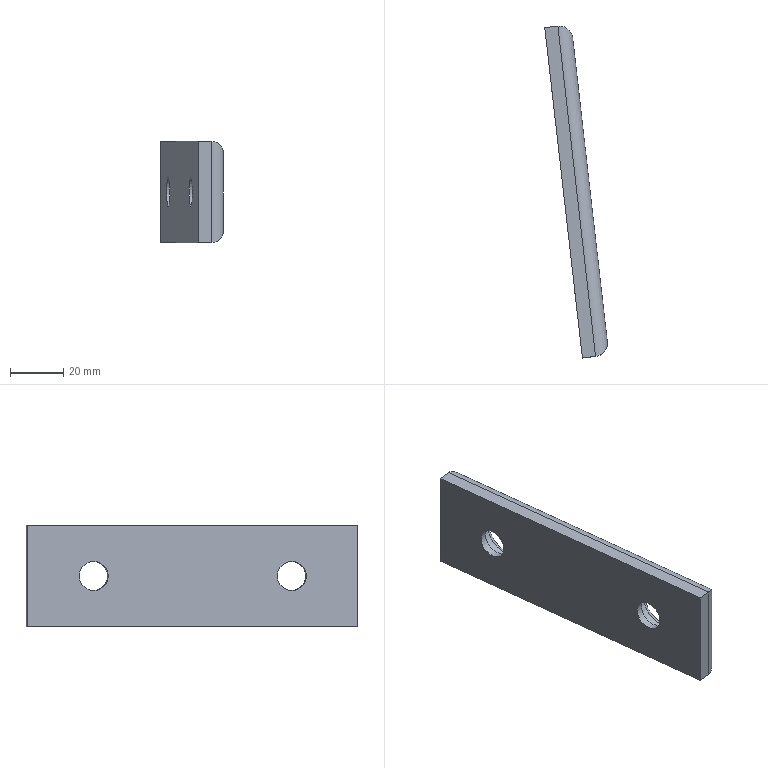Part | NX | features XQ 2 | 1 solid | 18 faces | box 23.552 x 124.795 x 38 mm | volume 41675 mm3 | plane 8 | cylinder 8 | torus 2 | commonest cylinder face diameters 10 x4 11 x2 17.5 x2
STEP:
#1=CARTESIAN_POINT('',(2947.085,251.295,-73.));
#2=VERTEX_POINT('',#1);
#3=CARTESIAN_POINT('',(2942.117,250.729,-73.));
#4=VERTEX_POINT('',#3);
#5=CARTESIAN_POINT('',(2947.085,251.295,-73.));
#6=DIRECTION('',(-0.9936,-0.1132,-0.000000001));
#7=VECTOR('',#6,1000.);
#8=LINE('',#5,#7);
#9=EDGE_CURVE('',#2,#4,#8,.T.);
#10=ORIENTED_EDGE('',*,*,#9,.F.);
#11=CARTESIAN_POINT('',(2947.085,251.295,-35.));
#12=VERTEX_POINT('',#11);
#13=CARTESIAN_POINT('',(2947.085,251.295,-54.));
#14=DIRECTION('',(0.000000001,0.,-1.));
#15=VECTOR('',#14,1000.);
#16=LINE('',#13,#15);
#17=EDGE_CURVE('',#12,#2,#16,.T.);
#18=ORIENTED_EDGE('',*,*,#17,.F.);
#19=CARTESIAN_POINT('',(2942.117,250.729,-35.));
#20=VERTEX_POINT('',#19);
#21=CARTESIAN_POINT('',(2947.085,251.295,-35.));
#22=DIRECTION('',(0.9936,0.1132,0.000000001));
#23=VECTOR('',#22,1000.);
#24=LINE('',#21,#23);
#25=EDGE_CURVE('',#20,#12,#24,.T.);
#26=ORIENTED_EDGE('',*,*,#25,.F.);
#27=CARTESIAN_POINT('',(2942.117,250.729,-59.));
#28=DIRECTION('',(0.000000001,0.,-1.));
#29=VECTOR('',#28,1000.);
#30=LINE('',#27,#29);
#31=EDGE_CURVE('',#20,#4,#30,.T.);
#32=ORIENTED_EDGE('',*,*,#31,.T.);
#33=EDGE_LOOP('',(#10,#18,#26,#32));
#34=FACE_BOUND('',#33,.T.);
#35=CARTESIAN_POINT('',(2947.085,251.295,-59.));
#36=DIRECTION('',(-0.1132,0.9936,0.));
#37=DIRECTION('',(0.9936,0.1132,0.000000001));
#38=AXIS2_PLACEMENT_3D('',#35,#36,#37);
#39=PLANE('',#38);
#40=ADVANCED_FACE('',(#34),#39,.F.);
#41=CARTESIAN_POINT('',(2927.967,374.925,-73.));
#42=VERTEX_POINT('',#41);
#43=CARTESIAN_POINT('',(2932.934,375.491,-73.));
#44=VERTEX_POINT('',#43);
#45=CARTESIAN_POINT('',(2932.934,375.491,-73.));
#46=DIRECTION('',(0.9936,0.1132,0.000000001));
#47=VECTOR('',#46,1000.);
#48=LINE('',#45,#47);
#49=EDGE_CURVE('',#42,#44,#48,.T.);
#50=ORIENTED_EDGE('',*,*,#49,.T.);
#51=CARTESIAN_POINT('',(2940.01,313.393,-73.));
#52=DIRECTION('',(-0.1132,0.9936,0.));
#53=VECTOR('',#52,1000.);
#54=LINE('',#51,#53);
#55=EDGE_CURVE('',#2,#44,#54,.T.);
#56=ORIENTED_EDGE('',*,*,#55,.F.);
#57=ORIENTED_EDGE('',*,*,#9,.T.);
#58=CARTESIAN_POINT('',(2935.042,312.827,-73.));
#59=DIRECTION('',(-0.1132,0.9936,0.));
#60=VECTOR('',#59,1000.);
#61=LINE('',#58,#60);
#62=EDGE_CURVE('',#4,#42,#61,.T.);
#63=ORIENTED_EDGE('',*,*,#62,.T.);
#64=EDGE_LOOP('',(#50,#56,#57,#63));
#65=FACE_BOUND('',#64,.T.);
#66=CARTESIAN_POINT('',(2940.01,313.393,-73.));
#67=DIRECTION('',(-0.000000001,0.,1.));
#68=DIRECTION('',(0.9936,0.1132,0.000000001));
#69=AXIS2_PLACEMENT_3D('',#66,#67,#68);
#70=PLANE('',#69);
#71=ADVANCED_FACE('',(#65),#70,.F.);
#72=ORIENTED_EDGE('',*,*,#55,.T.);
#73=CARTESIAN_POINT('',(2938.468,371.089,-68.));
#74=VERTEX_POINT('',#73);
#75=CARTESIAN_POINT('',(2933.5,370.523,-68.));
#76=DIRECTION('',(-0.08005,0.7026,0.7071));
#77=DIRECTION('',(0.08005,-0.7026,0.7071));
#78=AXIS2_PLACEMENT_3D('',#75,#76,#77);
#79=ELLIPSE('',#78,7.071,5.);
#80=EDGE_CURVE('',#74,#44,#79,.T.);
#81=ORIENTED_EDGE('',*,*,#80,.F.);
#82=CARTESIAN_POINT('',(2951.487,256.828,-68.));
#83=VERTEX_POINT('',#82);
#84=CARTESIAN_POINT('',(2944.977,313.959,-68.));
#85=DIRECTION('',(0.1132,-0.9936,0.));
#86=VECTOR('',#85,1000.);
#87=LINE('',#84,#86);
#88=EDGE_CURVE('',#74,#83,#87,.T.);
#89=ORIENTED_EDGE('',*,*,#88,.T.);
#90=CARTESIAN_POINT('',(2946.519,256.262,-68.));
#91=DIRECTION('',(-0.08005,0.7026,-0.7071));
#92=DIRECTION('',(-0.08005,0.7026,0.7071));
#93=AXIS2_PLACEMENT_3D('',#90,#91,#92);
#94=ELLIPSE('',#93,7.071,5.);
#95=EDGE_CURVE('',#83,#2,#94,.T.);
#96=ORIENTED_EDGE('',*,*,#95,.T.);
#97=EDGE_LOOP('',(#72,#81,#89,#96));
#98=FACE_BOUND('',#97,.T.);
#99=CARTESIAN_POINT('',(2940.01,313.393,-68.));
#100=DIRECTION('',(-0.1132,0.9936,0.));
#101=DIRECTION('',(0.7026,0.08005,-0.7071));
#102=AXIS2_PLACEMENT_3D('',#99,#100,#101);
#103=CYLINDRICAL_SURFACE('',#102,5.);
#104=ADVANCED_FACE('',(#98),#103,.T.);
#105=ORIENTED_EDGE('',*,*,#25,.T.);
#106=CARTESIAN_POINT('',(2932.934,375.491,-35.));
#107=VERTEX_POINT('',#106);
#108=CARTESIAN_POINT('',(2940.01,313.393,-35.));
#109=DIRECTION('',(0.1132,-0.9936,0.));
#110=VECTOR('',#109,1000.);
#111=LINE('',#108,#110);
#112=EDGE_CURVE('',#107,#12,#111,.T.);
#113=ORIENTED_EDGE('',*,*,#112,.F.);
#114=CARTESIAN_POINT('',(2927.967,374.925,-35.));
#115=VERTEX_POINT('',#114);
#116=CARTESIAN_POINT('',(2932.934,375.491,-35.));
#117=DIRECTION('',(-0.9936,-0.1132,-0.000000001));
#118=VECTOR('',#117,1000.);
#119=LINE('',#116,#118);
#120=EDGE_CURVE('',#107,#115,#119,.T.);
#121=ORIENTED_EDGE('',*,*,#120,.T.);
#122=CARTESIAN_POINT('',(2935.042,312.827,-35.));
#123=DIRECTION('',(0.1132,-0.9936,0.));
#124=VECTOR('',#123,1000.);
#125=LINE('',#122,#124);
#126=EDGE_CURVE('',#115,#20,#125,.T.);
#127=ORIENTED_EDGE('',*,*,#126,.T.);
#128=EDGE_LOOP('',(#105,#113,#121,#127));
#129=FACE_BOUND('',#128,.T.);
#130=CARTESIAN_POINT('',(2940.01,313.393,-35.));
#131=DIRECTION('',(0.000000001,0.,-1.));
#132=DIRECTION('',(-0.9936,-0.1132,-0.000000001));
#133=AXIS2_PLACEMENT_3D('',#130,#131,#132);
#134=PLANE('',#133);
#135=ADVANCED_FACE('',(#129),#134,.F.);
#136=CARTESIAN_POINT('',(2951.487,256.828,-40.));
#137=VERTEX_POINT('',#136);
#138=CARTESIAN_POINT('',(2938.468,371.089,-40.));
#139=VERTEX_POINT('',#138);
#140=CARTESIAN_POINT('',(2944.977,313.959,-40.));
#141=DIRECTION('',(-0.1132,0.9936,0.));
#142=VECTOR('',#141,1000.);
#143=LINE('',#140,#142);
#144=EDGE_CURVE('',#137,#139,#143,.T.);
#145=ORIENTED_EDGE('',*,*,#144,.T.);
#146=CARTESIAN_POINT('',(2933.5,370.523,-40.));
#147=DIRECTION('',(0.08005,-0.7026,0.7071));
#148=DIRECTION('',(0.08005,-0.7026,-0.7071));
#149=AXIS2_PLACEMENT_3D('',#146,#147,#148);
#150=ELLIPSE('',#149,7.071,5.);
#151=EDGE_CURVE('',#139,#107,#150,.T.);
#152=ORIENTED_EDGE('',*,*,#151,.T.);
#153=ORIENTED_EDGE('',*,*,#112,.T.);
#154=CARTESIAN_POINT('',(2946.519,256.262,-40.));
#155=DIRECTION('',(0.08005,-0.7026,-0.7071));
#156=DIRECTION('',(-0.08005,0.7026,-0.7071));
#157=AXIS2_PLACEMENT_3D('',#154,#155,#156);
#158=ELLIPSE('',#157,7.071,5.);
#159=EDGE_CURVE('',#137,#12,#158,.T.);
#160=ORIENTED_EDGE('',*,*,#159,.F.);
#161=EDGE_LOOP('',(#145,#152,#153,#160));
#162=FACE_BOUND('',#161,.T.);
#163=CARTESIAN_POINT('',(2940.01,313.393,-40.));
#164=DIRECTION('',(0.1132,-0.9936,0.));
#165=DIRECTION('',(0.7026,0.08005,0.7071));
#166=AXIS2_PLACEMENT_3D('',#163,#164,#165);
#167=CYLINDRICAL_SURFACE('',#166,5.);
#168=ADVANCED_FACE('',(#162),#167,.T.);
#169=ORIENTED_EDGE('',*,*,#17,.T.);
#170=ORIENTED_EDGE('',*,*,#95,.F.);
#171=CARTESIAN_POINT('',(2951.487,256.828,-54.));
#172=DIRECTION('',(-0.000000001,0.,1.));
#173=VECTOR('',#172,1000.);
#174=LINE('',#171,#173);
#175=EDGE_CURVE('',#83,#137,#174,.T.);
#176=ORIENTED_EDGE('',*,*,#175,.T.);
#177=ORIENTED_EDGE('',*,*,#159,.T.);
#178=EDGE_LOOP('',(#169,#170,#176,#177));
#179=FACE_BOUND('',#178,.T.);
#180=CARTESIAN_POINT('',(2946.519,256.262,-54.));
#181=DIRECTION('',(0.000000001,0.,-1.));
#182=DIRECTION('',(0.7826,-0.6225,0.000000001));
#183=AXIS2_PLACEMENT_3D('',#180,#181,#182);
#184=CYLINDRICAL_SURFACE('',#183,5.);
#185=ADVANCED_FACE('',(#179),#184,.T.);
#186=CARTESIAN_POINT('',(2938.468,371.089,-54.));
#187=DIRECTION('',(0.000000001,0.,-1.));
#188=VECTOR('',#187,1000.);
#189=LINE('',#186,#188);
#190=EDGE_CURVE('',#139,#74,#189,.T.);
#191=ORIENTED_EDGE('',*,*,#190,.T.);
#192=ORIENTED_EDGE('',*,*,#80,.T.);
#193=CARTESIAN_POINT('',(2932.934,375.491,-54.));
#194=DIRECTION('',(-0.000000001,0.,1.));
#195=VECTOR('',#194,1000.);
#196=LINE('',#193,#195);
#197=EDGE_CURVE('',#44,#107,#196,.T.);
#198=ORIENTED_EDGE('',*,*,#197,.T.);
#199=ORIENTED_EDGE('',*,*,#151,.F.);
#200=EDGE_LOOP('',(#191,#192,#198,#199));
#201=FACE_BOUND('',#200,.T.);
#202=CARTESIAN_POINT('',(2933.5,370.523,-54.));
#203=DIRECTION('',(-0.000000001,0.,1.));
#204=DIRECTION('',(0.6225,0.7826,0.));
#205=AXIS2_PLACEMENT_3D('',#202,#203,#204);
#206=CYLINDRICAL_SURFACE('',#205,5.);
#207=ADVANCED_FACE('',(#201),#206,.T.);
#208=CARTESIAN_POINT('',(2949.223,276.7,-64.75));
#209=VERTEX_POINT('',#208);
#210=CARTESIAN_POINT('',(2949.223,276.7,-54.));
#211=DIRECTION('',(0.9936,0.1132,0.000000001));
#212=DIRECTION('',(-0.000000001,0.,1.));
#213=AXIS2_PLACEMENT_3D('',#210,#211,#212);
#214=CIRCLE('',#213,10.75);
#215=EDGE_CURVE('',#209,#209,#214,.T.);
#216=ORIENTED_EDGE('',*,*,#215,.F.);
#217=EDGE_LOOP('',(#216));
#218=FACE_BOUND('',#217,.T.);
#219=ORIENTED_EDGE('',*,*,#190,.F.);
#220=ORIENTED_EDGE('',*,*,#144,.F.);
#221=ORIENTED_EDGE('',*,*,#175,.F.);
#222=ORIENTED_EDGE('',*,*,#88,.F.);
#223=EDGE_LOOP('',(#219,#220,#221,#222));
#224=FACE_BOUND('',#223,.T.);
#225=CARTESIAN_POINT('',(2940.732,351.218,-64.75));
#226=VERTEX_POINT('',#225);
#227=CARTESIAN_POINT('',(2940.732,351.218,-54.));
#228=DIRECTION('',(0.9936,0.1132,0.000000001));
#229=DIRECTION('',(-0.000000001,0.,1.));
#230=AXIS2_PLACEMENT_3D('',#227,#228,#229);
#231=CIRCLE('',#230,10.75);
#232=EDGE_CURVE('',#226,#226,#231,.T.);
#233=ORIENTED_EDGE('',*,*,#232,.F.);
#234=EDGE_LOOP('',(#233));
#235=FACE_BOUND('',#234,.T.);
#236=CARTESIAN_POINT('',(2944.977,313.959,-54.));
#237=DIRECTION('',(0.9936,0.1132,0.000000001));
#238=DIRECTION('',(0.000000001,0.,-1.));
#239=AXIS2_PLACEMENT_3D('',#236,#237,#238);
#240=PLANE('',#239);
#241=ADVANCED_FACE('',(#218,#224,#235),#240,.T.);
#242=ORIENTED_EDGE('',*,*,#31,.F.);
#243=ORIENTED_EDGE('',*,*,#126,.F.);
#244=CARTESIAN_POINT('',(2927.967,374.925,-59.));
#245=DIRECTION('',(0.000000001,0.,-1.));
#246=VECTOR('',#245,1000.);
#247=LINE('',#244,#246);
#248=EDGE_CURVE('',#115,#42,#247,.T.);
#249=ORIENTED_EDGE('',*,*,#248,.T.);
#250=ORIENTED_EDGE('',*,*,#62,.F.);
#251=EDGE_LOOP('',(#242,#243,#249,#250));
#252=FACE_BOUND('',#251,.T.);
#253=CARTESIAN_POINT('',(2939.287,275.568,-59.5));
#254=VERTEX_POINT('',#253);
#255=CARTESIAN_POINT('',(2939.287,275.568,-54.));
#256=DIRECTION('',(0.9936,0.1132,0.000000001));
#257=DIRECTION('',(0.000000001,0.,-1.));
#258=AXIS2_PLACEMENT_3D('',#255,#256,#257);
#259=CIRCLE('',#258,5.5);
#260=EDGE_CURVE('',#254,#254,#259,.T.);
#261=ORIENTED_EDGE('',*,*,#260,.T.);
#262=EDGE_LOOP('',(#261));
#263=FACE_BOUND('',#262,.T.);
#264=CARTESIAN_POINT('',(2930.797,350.086,-59.5));
#265=VERTEX_POINT('',#264);
#266=CARTESIAN_POINT('',(2930.797,350.086,-54.));
#267=DIRECTION('',(0.9936,0.1132,0.000000001));
#268=DIRECTION('',(0.000000001,0.,-1.));
#269=AXIS2_PLACEMENT_3D('',#266,#267,#268);
#270=CIRCLE('',#269,5.5);
#271=EDGE_CURVE('',#265,#265,#270,.T.);
#272=ORIENTED_EDGE('',*,*,#271,.T.);
#273=EDGE_LOOP('',(#272));
#274=FACE_BOUND('',#273,.T.);
#275=CARTESIAN_POINT('',(2935.042,312.827,-59.));
#276=DIRECTION('',(0.9936,0.1132,0.000000001));
#277=DIRECTION('',(0.000000001,0.,-1.));
#278=AXIS2_PLACEMENT_3D('',#275,#276,#277);
#279=PLANE('',#278);
#280=ADVANCED_FACE('',(#252,#263,#274),#279,.F.);
#281=CARTESIAN_POINT('',(2938.745,350.991,-62.75));
#282=VERTEX_POINT('',#281);
#283=CARTESIAN_POINT('',(2938.745,350.991,-54.));
#284=DIRECTION('',(-0.9936,-0.1132,-0.000000001));
#285=DIRECTION('',(-0.000000001,0.,1.));
#286=AXIS2_PLACEMENT_3D('',#283,#284,#285);
#287=CIRCLE('',#286,8.75);
#288=EDGE_CURVE('',#282,#282,#287,.T.);
#289=ORIENTED_EDGE('',*,*,#288,.T.);
#290=EDGE_LOOP('',(#289));
#291=FACE_BOUND('',#290,.T.);
#292=ORIENTED_EDGE('',*,*,#232,.T.);
#293=EDGE_LOOP('',(#292));
#294=FACE_BOUND('',#293,.T.);
#295=CARTESIAN_POINT('',(2938.745,350.991,-54.));
#296=DIRECTION('',(-0.9936,-0.1132,-0.000000001));
#297=DIRECTION('',(-0.000000001,0.,1.));
#298=AXIS2_PLACEMENT_3D('',#295,#296,#297);
#299=TOROIDAL_SURFACE('',#298,10.75,2.);
#300=ADVANCED_FACE('',(#291,#294),#299,.T.);
#301=CARTESIAN_POINT('',(2933.479,350.391,-62.75));
#302=VERTEX_POINT('',#301);
#303=CARTESIAN_POINT('',(2933.479,350.391,-54.));
#304=DIRECTION('',(-0.9936,-0.1132,-0.000000001));
#305=DIRECTION('',(0.000000001,0.,-1.));
#306=AXIS2_PLACEMENT_3D('',#303,#304,#305);
#307=CIRCLE('',#306,8.75);
#308=EDGE_CURVE('',#302,#302,#307,.T.);
#309=ORIENTED_EDGE('',*,*,#308,.T.);
#310=EDGE_LOOP('',(#309));
#311=FACE_BOUND('',#310,.T.);
#312=ORIENTED_EDGE('',*,*,#288,.F.);
#313=EDGE_LOOP('',(#312));
#314=FACE_BOUND('',#313,.T.);
#315=CARTESIAN_POINT('',(2937.106,350.805,-54.));
#316=DIRECTION('',(0.9936,0.1132,0.000000001));
#317=DIRECTION('',(0.000000001,0.,-1.));
#318=AXIS2_PLACEMENT_3D('',#315,#316,#317);
#319=CYLINDRICAL_SURFACE('',#318,8.75);
#320=ADVANCED_FACE('',(#311,#314),#319,.F.);
#321=CARTESIAN_POINT('',(2947.235,276.473,-62.75));
#322=VERTEX_POINT('',#321);
#323=CARTESIAN_POINT('',(2947.235,276.473,-54.));
#324=DIRECTION('',(-0.9936,-0.1132,-0.000000001));
#325=DIRECTION('',(-0.000000001,0.,1.));
#326=AXIS2_PLACEMENT_3D('',#323,#324,#325);
#327=CIRCLE('',#326,8.75);
#328=EDGE_CURVE('',#322,#322,#327,.T.);
#329=ORIENTED_EDGE('',*,*,#328,.T.);
#330=EDGE_LOOP('',(#329));
#331=FACE_BOUND('',#330,.T.);
#332=ORIENTED_EDGE('',*,*,#215,.T.);
#333=EDGE_LOOP('',(#332));
#334=FACE_BOUND('',#333,.T.);
#335=CARTESIAN_POINT('',(2947.235,276.473,-54.));
#336=DIRECTION('',(-0.9936,-0.1132,-0.000000001));
#337=DIRECTION('',(-0.000000001,0.,1.));
#338=AXIS2_PLACEMENT_3D('',#335,#336,#337);
#339=TOROIDAL_SURFACE('',#338,10.75,2.);
#340=ADVANCED_FACE('',(#331,#334),#339,.T.);
#341=CARTESIAN_POINT('',(2941.97,275.873,-62.75));
#342=VERTEX_POINT('',#341);
#343=CARTESIAN_POINT('',(2941.97,275.873,-54.));
#344=DIRECTION('',(-0.9936,-0.1132,-0.000000001));
#345=DIRECTION('',(0.000000001,0.,-1.));
#346=AXIS2_PLACEMENT_3D('',#343,#344,#345);
#347=CIRCLE('',#346,8.75);
#348=EDGE_CURVE('',#342,#342,#347,.T.);
#349=ORIENTED_EDGE('',*,*,#348,.T.);
#350=EDGE_LOOP('',(#349));
#351=FACE_BOUND('',#350,.T.);
#352=ORIENTED_EDGE('',*,*,#328,.F.);
#353=EDGE_LOOP('',(#352));
#354=FACE_BOUND('',#353,.T.);
#355=CARTESIAN_POINT('',(2945.596,276.287,-54.));
#356=DIRECTION('',(0.9936,0.1132,0.000000001));
#357=DIRECTION('',(0.000000001,0.,-1.));
#358=AXIS2_PLACEMENT_3D('',#355,#356,#357);
#359=CYLINDRICAL_SURFACE('',#358,8.75);
#360=ADVANCED_FACE('',(#351,#354),#359,.F.);
#361=ORIENTED_EDGE('',*,*,#271,.F.);
#362=EDGE_LOOP('',(#361));
#363=FACE_BOUND('',#362,.T.);
#364=CARTESIAN_POINT('',(2933.479,350.391,-59.5));
#365=VERTEX_POINT('',#364);
#366=CARTESIAN_POINT('',(2933.479,350.391,-54.));
#367=DIRECTION('',(0.9936,0.1132,0.000000001));
#368=DIRECTION('',(0.000000001,0.,-1.));
#369=AXIS2_PLACEMENT_3D('',#366,#367,#368);
#370=CIRCLE('',#369,5.5);
#371=EDGE_CURVE('',#365,#365,#370,.T.);
#372=ORIENTED_EDGE('',*,*,#371,.T.);
#373=EDGE_LOOP('',(#372));
#374=FACE_BOUND('',#373,.T.);
#375=CARTESIAN_POINT('',(2932.138,350.239,-54.));
#376=DIRECTION('',(0.9936,0.1132,0.000000001));
#377=DIRECTION('',(0.000000001,0.,-1.));
#378=AXIS2_PLACEMENT_3D('',#375,#376,#377);
#379=CYLINDRICAL_SURFACE('',#378,5.5);
#380=ADVANCED_FACE('',(#363,#374),#379,.F.);
#381=ORIENTED_EDGE('',*,*,#371,.F.);
#382=EDGE_LOOP('',(#381));
#383=FACE_BOUND('',#382,.T.);
#384=ORIENTED_EDGE('',*,*,#308,.F.);
#385=EDGE_LOOP('',(#384));
#386=FACE_BOUND('',#385,.T.);
#387=CARTESIAN_POINT('',(2933.479,350.391,-54.));
#388=DIRECTION('',(-0.9936,-0.1132,-0.000000001));
#389=DIRECTION('',(-0.000000001,0.,1.));
#390=AXIS2_PLACEMENT_3D('',#387,#388,#389);
#391=PLANE('',#390);
#392=ADVANCED_FACE('',(#383,#386),#391,.F.);
#393=ORIENTED_EDGE('',*,*,#260,.F.);
#394=EDGE_LOOP('',(#393));
#395=FACE_BOUND('',#394,.T.);
#396=CARTESIAN_POINT('',(2941.97,275.873,-59.5));
#397=VERTEX_POINT('',#396);
#398=CARTESIAN_POINT('',(2941.97,275.873,-54.));
#399=DIRECTION('',(0.9936,0.1132,0.000000001));
#400=DIRECTION('',(0.000000001,0.,-1.));
#401=AXIS2_PLACEMENT_3D('',#398,#399,#400);
#402=CIRCLE('',#401,5.5);
#403=EDGE_CURVE('',#397,#397,#402,.T.);
#404=ORIENTED_EDGE('',*,*,#403,.T.);
#405=EDGE_LOOP('',(#404));
#406=FACE_BOUND('',#405,.T.);
#407=CARTESIAN_POINT('',(2940.628,275.721,-54.));
#408=DIRECTION('',(0.9936,0.1132,0.000000001));
#409=DIRECTION('',(0.000000001,0.,-1.));
#410=AXIS2_PLACEMENT_3D('',#407,#408,#409);
#411=CYLINDRICAL_SURFACE('',#410,5.5);
#412=ADVANCED_FACE('',(#395,#406),#411,.F.);
#413=ORIENTED_EDGE('',*,*,#403,.F.);
#414=EDGE_LOOP('',(#413));
#415=FACE_BOUND('',#414,.T.);
#416=ORIENTED_EDGE('',*,*,#348,.F.);
#417=EDGE_LOOP('',(#416));
#418=FACE_BOUND('',#417,.T.);
#419=CARTESIAN_POINT('',(2941.97,275.873,-54.));
#420=DIRECTION('',(-0.9936,-0.1132,-0.000000001));
#421=DIRECTION('',(-0.000000001,0.,1.));
#422=AXIS2_PLACEMENT_3D('',#419,#420,#421);
#423=PLANE('',#422);
#424=ADVANCED_FACE('',(#415,#418),#423,.F.);
#425=ORIENTED_EDGE('',*,*,#197,.F.);
#426=ORIENTED_EDGE('',*,*,#49,.F.);
#427=ORIENTED_EDGE('',*,*,#248,.F.);
#428=ORIENTED_EDGE('',*,*,#120,.F.);
#429=EDGE_LOOP('',(#425,#426,#427,#428));
#430=FACE_BOUND('',#429,.T.);
#431=CARTESIAN_POINT('',(2932.934,375.491,-59.));
#432=DIRECTION('',(0.1132,-0.9936,0.));
#433=DIRECTION('',(-0.9936,-0.1132,-0.000000001));
#434=AXIS2_PLACEMENT_3D('',#431,#432,#433);
#435=PLANE('',#434);
#436=ADVANCED_FACE('',(#430),#435,.F.);
#437=CLOSED_SHELL('',(#40,#71,#104,#135,#168,#185,#207,#241,#280,#300,#320,#340,#360,#380,#392,#412,#424,#436));
#438=MANIFOLD_SOLID_BREP('',#437);
#439=(LENGTH_UNIT()NAMED_UNIT(*)SI_UNIT(.MILLI.,.METRE.));
#440=UNCERTAINTY_MEASURE_WITH_UNIT(LENGTH_MEASURE(0.00001),#439,'','');
#441=(NAMED_UNIT(*)PLANE_ANGLE_UNIT()SI_UNIT($,.RADIAN.));
#442=(NAMED_UNIT(*)SI_UNIT($,.STERADIAN.)SOLID_ANGLE_UNIT());
#443=(GEOMETRIC_REPRESENTATION_CONTEXT(3)GLOBAL_UNCERTAINTY_ASSIGNED_CONTEXT((#440))GLOBAL_UNIT_ASSIGNED_CONTEXT((#439,#441,#442))REPRESENTATION_CONTEXT('',''));
#444=ADVANCED_BREP_SHAPE_REPRESENTATION('',(#438),#443);